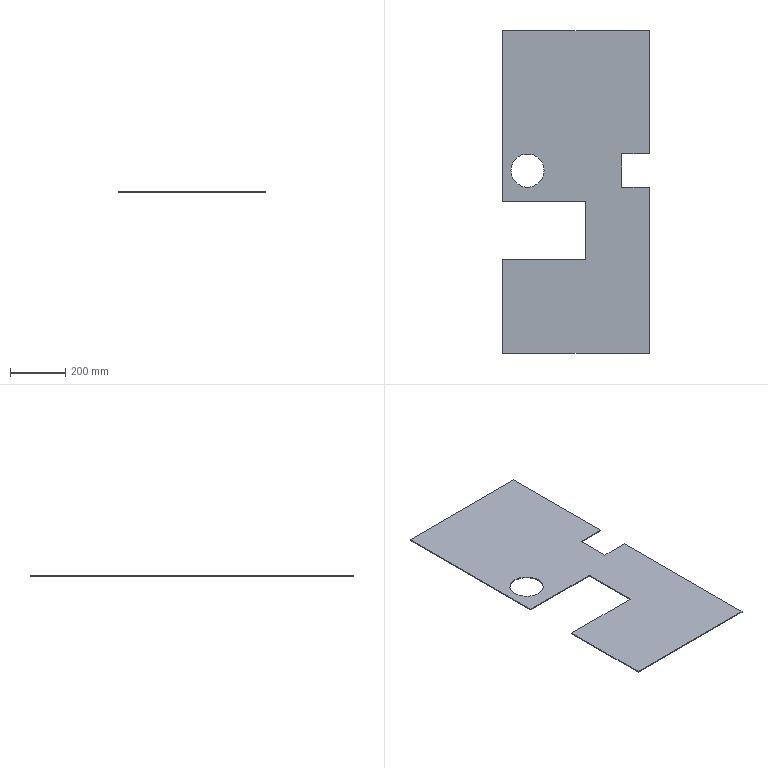Part | SolidWorks | features Extrusion 1, ICE 1 | 1 solid | 16 faces | box 530 x 1165 x 3 mm | volume 1593421 mm3 | plane 14 | cylinder 2 | commonest cylinder face diameters 120 x2
STEP:
#1=CARTESIAN_POINT('',(150.,660.,3.));
#2=VERTEX_POINT('',#1);
#3=CARTESIAN_POINT('',(30.,660.,3.));
#4=VERTEX_POINT('',#3);
#5=CARTESIAN_POINT('',(90.,660.,3.));
#6=DIRECTION('',(0.,0.,-1.));
#7=DIRECTION('',(-1.,0.,0.));
#8=AXIS2_PLACEMENT_3D('',#5,#6,#7);
#9=CIRCLE('',#8,60.);
#10=EDGE_CURVE('',#2,#4,#9,.T.);
#11=ORIENTED_EDGE('',*,*,#10,.F.);
#12=CARTESIAN_POINT('',(150.,660.,0.));
#13=VERTEX_POINT('',#12);
#14=CARTESIAN_POINT('',(150.,660.,10.));
#15=DIRECTION('',(0.,0.,-1.));
#16=VECTOR('',#15,1000.);
#17=LINE('',#14,#16);
#18=EDGE_CURVE('',#2,#13,#17,.T.);
#19=ORIENTED_EDGE('',*,*,#18,.T.);
#20=CARTESIAN_POINT('',(30.,660.,0.));
#21=VERTEX_POINT('',#20);
#22=CARTESIAN_POINT('',(90.,660.,0.));
#23=DIRECTION('',(0.,0.,-1.));
#24=DIRECTION('',(-1.,0.,0.));
#25=AXIS2_PLACEMENT_3D('',#22,#23,#24);
#26=CIRCLE('',#25,60.);
#27=EDGE_CURVE('',#13,#21,#26,.T.);
#28=ORIENTED_EDGE('',*,*,#27,.T.);
#29=CARTESIAN_POINT('',(30.,660.,10.));
#30=DIRECTION('',(0.,0.,-1.));
#31=VECTOR('',#30,1000.);
#32=LINE('',#29,#31);
#33=EDGE_CURVE('',#4,#21,#32,.T.);
#34=ORIENTED_EDGE('',*,*,#33,.F.);
#35=EDGE_LOOP('',(#11,#19,#28,#34));
#36=FACE_OUTER_BOUND('',#35,.T.);
#37=CARTESIAN_POINT('',(90.,660.,10.));
#38=DIRECTION('',(0.,0.,-1.));
#39=DIRECTION('',(-1.,0.,0.));
#40=AXIS2_PLACEMENT_3D('',#37,#38,#39);
#41=CYLINDRICAL_SURFACE('',#40,60.);
#42=ADVANCED_FACE('',(#36),#41,.F.);
#43=CARTESIAN_POINT('',(530.,720.,3.));
#44=VERTEX_POINT('',#43);
#45=CARTESIAN_POINT('',(530.,1165.,3.));
#46=VERTEX_POINT('',#45);
#47=CARTESIAN_POINT('',(530.,0.,3.));
#48=DIRECTION('',(0.,1.,0.));
#49=VECTOR('',#48,1000.);
#50=LINE('',#47,#49);
#51=EDGE_CURVE('',#44,#46,#50,.T.);
#52=ORIENTED_EDGE('',*,*,#51,.F.);
#53=CARTESIAN_POINT('',(530.,720.,0.));
#54=VERTEX_POINT('',#53);
#55=CARTESIAN_POINT('',(530.,720.,3.));
#56=DIRECTION('',(0.,0.,-1.));
#57=VECTOR('',#56,1000.);
#58=LINE('',#55,#57);
#59=EDGE_CURVE('',#44,#54,#58,.T.);
#60=ORIENTED_EDGE('',*,*,#59,.T.);
#61=CARTESIAN_POINT('',(530.,1165.,0.));
#62=VERTEX_POINT('',#61);
#63=CARTESIAN_POINT('',(530.,0.,0.));
#64=DIRECTION('',(0.,1.,0.));
#65=VECTOR('',#64,1000.);
#66=LINE('',#63,#65);
#67=EDGE_CURVE('',#54,#62,#66,.T.);
#68=ORIENTED_EDGE('',*,*,#67,.T.);
#69=CARTESIAN_POINT('',(530.,1165.,3.));
#70=DIRECTION('',(0.,0.,-1.));
#71=VECTOR('',#70,1000.);
#72=LINE('',#69,#71);
#73=EDGE_CURVE('',#46,#62,#72,.T.);
#74=ORIENTED_EDGE('',*,*,#73,.F.);
#75=EDGE_LOOP('',(#52,#60,#68,#74));
#76=FACE_OUTER_BOUND('',#75,.T.);
#77=CARTESIAN_POINT('',(530.,0.,3.));
#78=DIRECTION('',(-1.,0.,0.));
#79=DIRECTION('',(0.,-1.,0.));
#80=AXIS2_PLACEMENT_3D('',#77,#78,#79);
#81=PLANE('',#80);
#82=ADVANCED_FACE('',(#76),#81,.F.);
#83=CARTESIAN_POINT('',(0.,340.,0.));
#84=VERTEX_POINT('',#83);
#85=CARTESIAN_POINT('',(0.,0.,0.));
#86=VERTEX_POINT('',#85);
#87=CARTESIAN_POINT('',(0.,0.,0.));
#88=DIRECTION('',(0.,-1.,0.));
#89=VECTOR('',#88,1000.);
#90=LINE('',#87,#89);
#91=EDGE_CURVE('',#84,#86,#90,.T.);
#92=ORIENTED_EDGE('',*,*,#91,.T.);
#93=CARTESIAN_POINT('',(0.,0.,3.));
#94=VERTEX_POINT('',#93);
#95=CARTESIAN_POINT('',(0.,0.,3.));
#96=DIRECTION('',(0.,0.,-1.));
#97=VECTOR('',#96,1000.);
#98=LINE('',#95,#97);
#99=EDGE_CURVE('',#94,#86,#98,.T.);
#100=ORIENTED_EDGE('',*,*,#99,.F.);
#101=CARTESIAN_POINT('',(0.,340.,3.));
#102=VERTEX_POINT('',#101);
#103=CARTESIAN_POINT('',(0.,0.,3.));
#104=DIRECTION('',(0.,-1.,0.));
#105=VECTOR('',#104,1000.);
#106=LINE('',#103,#105);
#107=EDGE_CURVE('',#102,#94,#106,.T.);
#108=ORIENTED_EDGE('',*,*,#107,.F.);
#109=CARTESIAN_POINT('',(0.,340.,3.));
#110=DIRECTION('',(0.,0.,-1.));
#111=VECTOR('',#110,1000.);
#112=LINE('',#109,#111);
#113=EDGE_CURVE('',#102,#84,#112,.T.);
#114=ORIENTED_EDGE('',*,*,#113,.T.);
#115=EDGE_LOOP('',(#92,#100,#108,#114));
#116=FACE_OUTER_BOUND('',#115,.T.);
#117=CARTESIAN_POINT('',(0.,0.,3.));
#118=DIRECTION('',(1.,0.,0.));
#119=DIRECTION('',(0.,0.,-1.));
#120=AXIS2_PLACEMENT_3D('',#117,#118,#119);
#121=PLANE('',#120);
#122=ADVANCED_FACE('',(#116),#121,.F.);
#123=CARTESIAN_POINT('',(530.,0.,0.));
#124=VERTEX_POINT('',#123);
#125=CARTESIAN_POINT('',(0.,0.,0.));
#126=DIRECTION('',(1.,0.,0.));
#127=VECTOR('',#126,1000.);
#128=LINE('',#125,#127);
#129=EDGE_CURVE('',#86,#124,#128,.T.);
#130=ORIENTED_EDGE('',*,*,#129,.T.);
#131=CARTESIAN_POINT('',(530.,0.,3.));
#132=VERTEX_POINT('',#131);
#133=CARTESIAN_POINT('',(530.,0.,3.));
#134=DIRECTION('',(0.,0.,-1.));
#135=VECTOR('',#134,1000.);
#136=LINE('',#133,#135);
#137=EDGE_CURVE('',#132,#124,#136,.T.);
#138=ORIENTED_EDGE('',*,*,#137,.F.);
#139=CARTESIAN_POINT('',(0.,0.,3.));
#140=DIRECTION('',(1.,0.,0.));
#141=VECTOR('',#140,1000.);
#142=LINE('',#139,#141);
#143=EDGE_CURVE('',#94,#132,#142,.T.);
#144=ORIENTED_EDGE('',*,*,#143,.F.);
#145=ORIENTED_EDGE('',*,*,#99,.T.);
#146=EDGE_LOOP('',(#130,#138,#144,#145));
#147=FACE_OUTER_BOUND('',#146,.T.);
#148=CARTESIAN_POINT('',(0.,0.,3.));
#149=DIRECTION('',(0.,1.,0.));
#150=DIRECTION('',(0.,0.,1.));
#151=AXIS2_PLACEMENT_3D('',#148,#149,#150);
#152=PLANE('',#151);
#153=ADVANCED_FACE('',(#147),#152,.F.);
#154=CARTESIAN_POINT('',(530.,600.,0.));
#155=VERTEX_POINT('',#154);
#156=CARTESIAN_POINT('',(530.,0.,0.));
#157=DIRECTION('',(0.,1.,0.));
#158=VECTOR('',#157,1000.);
#159=LINE('',#156,#158);
#160=EDGE_CURVE('',#124,#155,#159,.T.);
#161=ORIENTED_EDGE('',*,*,#160,.T.);
#162=CARTESIAN_POINT('',(530.,600.,3.));
#163=VERTEX_POINT('',#162);
#164=CARTESIAN_POINT('',(530.,600.,3.));
#165=DIRECTION('',(0.,0.,1.));
#166=VECTOR('',#165,1000.);
#167=LINE('',#164,#166);
#168=EDGE_CURVE('',#155,#163,#167,.T.);
#169=ORIENTED_EDGE('',*,*,#168,.T.);
#170=CARTESIAN_POINT('',(530.,0.,3.));
#171=DIRECTION('',(0.,1.,0.));
#172=VECTOR('',#171,1000.);
#173=LINE('',#170,#172);
#174=EDGE_CURVE('',#132,#163,#173,.T.);
#175=ORIENTED_EDGE('',*,*,#174,.F.);
#176=ORIENTED_EDGE('',*,*,#137,.T.);
#177=EDGE_LOOP('',(#161,#169,#175,#176));
#178=FACE_OUTER_BOUND('',#177,.T.);
#179=CARTESIAN_POINT('',(530.,0.,3.));
#180=DIRECTION('',(-1.,0.,0.));
#181=DIRECTION('',(0.,-1.,0.));
#182=AXIS2_PLACEMENT_3D('',#179,#180,#181);
#183=PLANE('',#182);
#184=ADVANCED_FACE('',(#178),#183,.F.);
#185=CARTESIAN_POINT('',(0.,1165.,0.));
#186=VERTEX_POINT('',#185);
#187=CARTESIAN_POINT('',(0.,1165.,0.));
#188=DIRECTION('',(-1.,0.,0.));
#189=VECTOR('',#188,1000.);
#190=LINE('',#187,#189);
#191=EDGE_CURVE('',#62,#186,#190,.T.);
#192=ORIENTED_EDGE('',*,*,#191,.T.);
#193=CARTESIAN_POINT('',(0.,1165.,3.));
#194=VERTEX_POINT('',#193);
#195=CARTESIAN_POINT('',(0.,1165.,3.));
#196=DIRECTION('',(0.,0.,-1.));
#197=VECTOR('',#196,1000.);
#198=LINE('',#195,#197);
#199=EDGE_CURVE('',#194,#186,#198,.T.);
#200=ORIENTED_EDGE('',*,*,#199,.F.);
#201=CARTESIAN_POINT('',(0.,1165.,3.));
#202=DIRECTION('',(-1.,0.,0.));
#203=VECTOR('',#202,1000.);
#204=LINE('',#201,#203);
#205=EDGE_CURVE('',#46,#194,#204,.T.);
#206=ORIENTED_EDGE('',*,*,#205,.F.);
#207=ORIENTED_EDGE('',*,*,#73,.T.);
#208=EDGE_LOOP('',(#192,#200,#206,#207));
#209=FACE_OUTER_BOUND('',#208,.T.);
#210=CARTESIAN_POINT('',(0.,1165.,3.));
#211=DIRECTION('',(0.,-1.,0.));
#212=DIRECTION('',(0.,0.,-1.));
#213=AXIS2_PLACEMENT_3D('',#210,#211,#212);
#214=PLANE('',#213);
#215=ADVANCED_FACE('',(#209),#214,.F.);
#216=CARTESIAN_POINT('',(0.,550.,0.));
#217=VERTEX_POINT('',#216);
#218=CARTESIAN_POINT('',(0.,550.,0.));
#219=DIRECTION('',(0.,-1.,0.));
#220=VECTOR('',#219,1000.);
#221=LINE('',#218,#220);
#222=EDGE_CURVE('',#186,#217,#221,.T.);
#223=ORIENTED_EDGE('',*,*,#222,.T.);
#224=CARTESIAN_POINT('',(0.,550.,3.));
#225=VERTEX_POINT('',#224);
#226=CARTESIAN_POINT('',(0.,550.,3.));
#227=DIRECTION('',(0.,0.,-1.));
#228=VECTOR('',#227,1000.);
#229=LINE('',#226,#228);
#230=EDGE_CURVE('',#225,#217,#229,.T.);
#231=ORIENTED_EDGE('',*,*,#230,.F.);
#232=CARTESIAN_POINT('',(0.,550.,3.));
#233=DIRECTION('',(0.,-1.,0.));
#234=VECTOR('',#233,1000.);
#235=LINE('',#232,#234);
#236=EDGE_CURVE('',#194,#225,#235,.T.);
#237=ORIENTED_EDGE('',*,*,#236,.F.);
#238=ORIENTED_EDGE('',*,*,#199,.T.);
#239=EDGE_LOOP('',(#223,#231,#237,#238));
#240=FACE_OUTER_BOUND('',#239,.T.);
#241=CARTESIAN_POINT('',(0.,550.,3.));
#242=DIRECTION('',(1.,0.,0.));
#243=DIRECTION('',(0.,1.,0.));
#244=AXIS2_PLACEMENT_3D('',#241,#242,#243);
#245=PLANE('',#244);
#246=ADVANCED_FACE('',(#240),#245,.F.);
#247=CARTESIAN_POINT('',(300.,550.,0.));
#248=VERTEX_POINT('',#247);
#249=CARTESIAN_POINT('',(300.,550.,0.));
#250=DIRECTION('',(1.,0.,0.));
#251=VECTOR('',#250,1000.);
#252=LINE('',#249,#251);
#253=EDGE_CURVE('',#217,#248,#252,.T.);
#254=ORIENTED_EDGE('',*,*,#253,.T.);
#255=CARTESIAN_POINT('',(300.,550.,3.));
#256=VERTEX_POINT('',#255);
#257=CARTESIAN_POINT('',(300.,550.,3.));
#258=DIRECTION('',(0.,0.,-1.));
#259=VECTOR('',#258,1000.);
#260=LINE('',#257,#259);
#261=EDGE_CURVE('',#256,#248,#260,.T.);
#262=ORIENTED_EDGE('',*,*,#261,.F.);
#263=CARTESIAN_POINT('',(300.,550.,3.));
#264=DIRECTION('',(1.,0.,0.));
#265=VECTOR('',#264,1000.);
#266=LINE('',#263,#265);
#267=EDGE_CURVE('',#225,#256,#266,.T.);
#268=ORIENTED_EDGE('',*,*,#267,.F.);
#269=ORIENTED_EDGE('',*,*,#230,.T.);
#270=EDGE_LOOP('',(#254,#262,#268,#269));
#271=FACE_OUTER_BOUND('',#270,.T.);
#272=CARTESIAN_POINT('',(300.,550.,3.));
#273=DIRECTION('',(0.,1.,0.));
#274=DIRECTION('',(0.,0.,1.));
#275=AXIS2_PLACEMENT_3D('',#272,#273,#274);
#276=PLANE('',#275);
#277=ADVANCED_FACE('',(#271),#276,.F.);
#278=CARTESIAN_POINT('',(300.,340.,0.));
#279=VERTEX_POINT('',#278);
#280=CARTESIAN_POINT('',(300.,340.,0.));
#281=DIRECTION('',(0.,-1.,0.));
#282=VECTOR('',#281,1000.);
#283=LINE('',#280,#282);
#284=EDGE_CURVE('',#248,#279,#283,.T.);
#285=ORIENTED_EDGE('',*,*,#284,.T.);
#286=CARTESIAN_POINT('',(300.,340.,3.));
#287=VERTEX_POINT('',#286);
#288=CARTESIAN_POINT('',(300.,340.,3.));
#289=DIRECTION('',(0.,0.,-1.));
#290=VECTOR('',#289,1000.);
#291=LINE('',#288,#290);
#292=EDGE_CURVE('',#287,#279,#291,.T.);
#293=ORIENTED_EDGE('',*,*,#292,.F.);
#294=CARTESIAN_POINT('',(300.,340.,3.));
#295=DIRECTION('',(0.,-1.,0.));
#296=VECTOR('',#295,1000.);
#297=LINE('',#294,#296);
#298=EDGE_CURVE('',#256,#287,#297,.T.);
#299=ORIENTED_EDGE('',*,*,#298,.F.);
#300=ORIENTED_EDGE('',*,*,#261,.T.);
#301=EDGE_LOOP('',(#285,#293,#299,#300));
#302=FACE_OUTER_BOUND('',#301,.T.);
#303=CARTESIAN_POINT('',(300.,340.,3.));
#304=DIRECTION('',(1.,0.,0.));
#305=DIRECTION('',(0.,0.,-1.));
#306=AXIS2_PLACEMENT_3D('',#303,#304,#305);
#307=PLANE('',#306);
#308=ADVANCED_FACE('',(#302),#307,.F.);
#309=CARTESIAN_POINT('',(0.,340.,0.));
#310=DIRECTION('',(-1.,0.,0.));
#311=VECTOR('',#310,1000.);
#312=LINE('',#309,#311);
#313=EDGE_CURVE('',#279,#84,#312,.T.);
#314=ORIENTED_EDGE('',*,*,#313,.T.);
#315=ORIENTED_EDGE('',*,*,#113,.F.);
#316=CARTESIAN_POINT('',(0.,340.,3.));
#317=DIRECTION('',(-1.,0.,0.));
#318=VECTOR('',#317,1000.);
#319=LINE('',#316,#318);
#320=EDGE_CURVE('',#287,#102,#319,.T.);
#321=ORIENTED_EDGE('',*,*,#320,.F.);
#322=ORIENTED_EDGE('',*,*,#292,.T.);
#323=EDGE_LOOP('',(#314,#315,#321,#322));
#324=FACE_OUTER_BOUND('',#323,.T.);
#325=CARTESIAN_POINT('',(0.,340.,3.));
#326=DIRECTION('',(0.,-1.,0.));
#327=DIRECTION('',(0.,0.,-1.));
#328=AXIS2_PLACEMENT_3D('',#325,#326,#327);
#329=PLANE('',#328);
#330=ADVANCED_FACE('',(#324),#329,.F.);
#331=CARTESIAN_POINT('',(90.,660.,3.));
#332=DIRECTION('',(0.,0.,-1.));
#333=DIRECTION('',(-1.,0.,0.));
#334=AXIS2_PLACEMENT_3D('',#331,#332,#333);
#335=CIRCLE('',#334,60.);
#336=EDGE_CURVE('',#4,#2,#335,.T.);
#337=ORIENTED_EDGE('',*,*,#336,.T.);
#338=ORIENTED_EDGE('',*,*,#10,.T.);
#339=EDGE_LOOP('',(#337,#338));
#340=FACE_BOUND('',#339,.T.);
#341=CARTESIAN_POINT('',(430.,600.,3.));
#342=VERTEX_POINT('',#341);
#343=CARTESIAN_POINT('',(430.,720.,3.));
#344=VERTEX_POINT('',#343);
#345=CARTESIAN_POINT('',(430.,0.,3.));
#346=DIRECTION('',(0.,1.,0.));
#347=VECTOR('',#346,1000.);
#348=LINE('',#345,#347);
#349=EDGE_CURVE('',#342,#344,#348,.T.);
#350=ORIENTED_EDGE('',*,*,#349,.T.);
#351=CARTESIAN_POINT('',(0.,720.,3.));
#352=DIRECTION('',(1.,0.,0.));
#353=VECTOR('',#352,1000.);
#354=LINE('',#351,#353);
#355=EDGE_CURVE('',#344,#44,#354,.T.);
#356=ORIENTED_EDGE('',*,*,#355,.T.);
#357=ORIENTED_EDGE('',*,*,#51,.T.);
#358=ORIENTED_EDGE('',*,*,#205,.T.);
#359=ORIENTED_EDGE('',*,*,#236,.T.);
#360=ORIENTED_EDGE('',*,*,#267,.T.);
#361=ORIENTED_EDGE('',*,*,#298,.T.);
#362=ORIENTED_EDGE('',*,*,#320,.T.);
#363=ORIENTED_EDGE('',*,*,#107,.T.);
#364=ORIENTED_EDGE('',*,*,#143,.T.);
#365=ORIENTED_EDGE('',*,*,#174,.T.);
#366=CARTESIAN_POINT('',(0.,600.,3.));
#367=DIRECTION('',(-1.,0.,0.));
#368=VECTOR('',#367,1000.);
#369=LINE('',#366,#368);
#370=EDGE_CURVE('',#163,#342,#369,.T.);
#371=ORIENTED_EDGE('',*,*,#370,.T.);
#372=EDGE_LOOP('',(#350,#356,#357,#358,#359,#360,#361,#362,#363,#364,#365,#371));
#373=FACE_OUTER_BOUND('',#372,.T.);
#374=CARTESIAN_POINT('',(0.,0.,3.));
#375=DIRECTION('',(0.,0.,-1.));
#376=DIRECTION('',(-1.,0.,0.));
#377=AXIS2_PLACEMENT_3D('',#374,#375,#376);
#378=PLANE('',#377);
#379=ADVANCED_FACE('',(#340,#373),#378,.F.);
#380=CARTESIAN_POINT('',(430.,720.,0.));
#381=VERTEX_POINT('',#380);
#382=CARTESIAN_POINT('',(430.,720.,0.));
#383=DIRECTION('',(1.,0.,0.));
#384=VECTOR('',#383,1000.);
#385=LINE('',#382,#384);
#386=EDGE_CURVE('',#381,#54,#385,.T.);
#387=ORIENTED_EDGE('',*,*,#386,.F.);
#388=CARTESIAN_POINT('',(430.,600.,0.));
#389=VERTEX_POINT('',#388);
#390=CARTESIAN_POINT('',(430.,600.,0.));
#391=DIRECTION('',(0.,1.,0.));
#392=VECTOR('',#391,1000.);
#393=LINE('',#390,#392);
#394=EDGE_CURVE('',#389,#381,#393,.T.);
#395=ORIENTED_EDGE('',*,*,#394,.F.);
#396=CARTESIAN_POINT('',(0.,600.,0.));
#397=DIRECTION('',(-1.,0.,0.));
#398=VECTOR('',#397,1000.);
#399=LINE('',#396,#398);
#400=EDGE_CURVE('',#155,#389,#399,.T.);
#401=ORIENTED_EDGE('',*,*,#400,.F.);
#402=ORIENTED_EDGE('',*,*,#160,.F.);
#403=ORIENTED_EDGE('',*,*,#129,.F.);
#404=ORIENTED_EDGE('',*,*,#91,.F.);
#405=ORIENTED_EDGE('',*,*,#313,.F.);
#406=ORIENTED_EDGE('',*,*,#284,.F.);
#407=ORIENTED_EDGE('',*,*,#253,.F.);
#408=ORIENTED_EDGE('',*,*,#222,.F.);
#409=ORIENTED_EDGE('',*,*,#191,.F.);
#410=ORIENTED_EDGE('',*,*,#67,.F.);
#411=EDGE_LOOP('',(#387,#395,#401,#402,#403,#404,#405,#406,#407,#408,#409,#410));
#412=FACE_OUTER_BOUND('',#411,.T.);
#413=CARTESIAN_POINT('',(90.,660.,0.));
#414=DIRECTION('',(0.,0.,-1.));
#415=DIRECTION('',(-1.,0.,0.));
#416=AXIS2_PLACEMENT_3D('',#413,#414,#415);
#417=CIRCLE('',#416,60.);
#418=EDGE_CURVE('',#21,#13,#417,.T.);
#419=ORIENTED_EDGE('',*,*,#418,.F.);
#420=ORIENTED_EDGE('',*,*,#27,.F.);
#421=EDGE_LOOP('',(#419,#420));
#422=FACE_BOUND('',#421,.T.);
#423=CARTESIAN_POINT('',(0.,0.,0.));
#424=DIRECTION('',(0.,0.,-1.));
#425=DIRECTION('',(-1.,0.,0.));
#426=AXIS2_PLACEMENT_3D('',#423,#424,#425);
#427=PLANE('',#426);
#428=ADVANCED_FACE('',(#412,#422),#427,.T.);
#429=ORIENTED_EDGE('',*,*,#18,.F.);
#430=ORIENTED_EDGE('',*,*,#336,.F.);
#431=ORIENTED_EDGE('',*,*,#33,.T.);
#432=ORIENTED_EDGE('',*,*,#418,.T.);
#433=EDGE_LOOP('',(#429,#430,#431,#432));
#434=FACE_OUTER_BOUND('',#433,.T.);
#435=CARTESIAN_POINT('',(90.,660.,10.));
#436=DIRECTION('',(0.,0.,-1.));
#437=DIRECTION('',(-1.,0.,0.));
#438=AXIS2_PLACEMENT_3D('',#435,#436,#437);
#439=CYLINDRICAL_SURFACE('',#438,60.);
#440=ADVANCED_FACE('',(#434),#439,.F.);
#441=ORIENTED_EDGE('',*,*,#355,.F.);
#442=CARTESIAN_POINT('',(430.,720.,10.));
#443=DIRECTION('',(0.,0.,-1.));
#444=VECTOR('',#443,1000.);
#445=LINE('',#442,#444);
#446=EDGE_CURVE('',#344,#381,#445,.T.);
#447=ORIENTED_EDGE('',*,*,#446,.T.);
#448=ORIENTED_EDGE('',*,*,#386,.T.);
#449=ORIENTED_EDGE('',*,*,#59,.F.);
#450=EDGE_LOOP('',(#441,#447,#448,#449));
#451=FACE_OUTER_BOUND('',#450,.T.);
#452=CARTESIAN_POINT('',(430.,720.,10.));
#453=DIRECTION('',(0.,1.,0.));
#454=DIRECTION('',(0.,0.,1.));
#455=AXIS2_PLACEMENT_3D('',#452,#453,#454);
#456=PLANE('',#455);
#457=ADVANCED_FACE('',(#451),#456,.F.);
#458=CARTESIAN_POINT('',(430.,600.,10.));
#459=DIRECTION('',(0.,0.,-1.));
#460=VECTOR('',#459,1000.);
#461=LINE('',#458,#460);
#462=EDGE_CURVE('',#342,#389,#461,.T.);
#463=ORIENTED_EDGE('',*,*,#462,.T.);
#464=ORIENTED_EDGE('',*,*,#394,.T.);
#465=ORIENTED_EDGE('',*,*,#446,.F.);
#466=ORIENTED_EDGE('',*,*,#349,.F.);
#467=EDGE_LOOP('',(#463,#464,#465,#466));
#468=FACE_OUTER_BOUND('',#467,.T.);
#469=CARTESIAN_POINT('',(430.,600.,10.));
#470=DIRECTION('',(-1.,0.,0.));
#471=DIRECTION('',(0.,0.,1.));
#472=AXIS2_PLACEMENT_3D('',#469,#470,#471);
#473=PLANE('',#472);
#474=ADVANCED_FACE('',(#468),#473,.F.);
#475=ORIENTED_EDGE('',*,*,#400,.T.);
#476=ORIENTED_EDGE('',*,*,#462,.F.);
#477=ORIENTED_EDGE('',*,*,#370,.F.);
#478=ORIENTED_EDGE('',*,*,#168,.F.);
#479=EDGE_LOOP('',(#475,#476,#477,#478));
#480=FACE_OUTER_BOUND('',#479,.T.);
#481=CARTESIAN_POINT('',(430.,600.,10.));
#482=DIRECTION('',(0.,-1.,0.));
#483=DIRECTION('',(0.,0.,-1.));
#484=AXIS2_PLACEMENT_3D('',#481,#482,#483);
#485=PLANE('',#484);
#486=ADVANCED_FACE('',(#480),#485,.F.);
#487=CLOSED_SHELL('',(#42,#82,#122,#153,#184,#215,#246,#277,#308,#330,#379,#428,#440,#457,#474,#486));
#488=MANIFOLD_SOLID_BREP('',#487);
#489=CARTESIAN_POINT('',(0.,0.,0.));
#490=DIRECTION('',(0.,0.,1.));
#491=DIRECTION('',(1.,0.,0.));
#492=AXIS2_PLACEMENT_3D('',#489,#490,#491);
#493=(LENGTH_UNIT()NAMED_UNIT(*)SI_UNIT(.MILLI.,.METRE.));
#494=UNCERTAINTY_MEASURE_WITH_UNIT(LENGTH_MEASURE(0.00001),#493,'','');
#495=(NAMED_UNIT(*)PLANE_ANGLE_UNIT()SI_UNIT($,.RADIAN.));
#496=(NAMED_UNIT(*)SI_UNIT($,.STERADIAN.)SOLID_ANGLE_UNIT());
#497=(GEOMETRIC_REPRESENTATION_CONTEXT(3)GLOBAL_UNCERTAINTY_ASSIGNED_CONTEXT((#494))GLOBAL_UNIT_ASSIGNED_CONTEXT((#493,#495,#496))REPRESENTATION_CONTEXT('',''));
#498=ADVANCED_BREP_SHAPE_REPRESENTATION('',(#488,#492),#497);